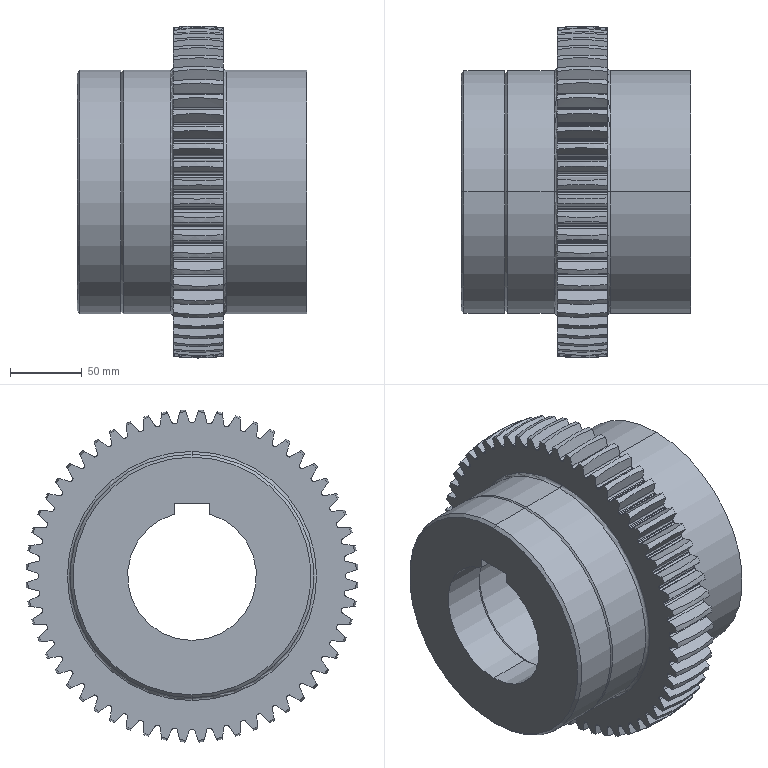Part | STEP file | External ring gear m=4  Z=56 | 1 solid | 391 faces | box 160.5 x 231.789 x 231.789 mm | volume 3084589 mm3 | cylinder 202 | spline 112 | sphere 56 | plane 10 | cone 7 | torus 4 | commonest cylinder face diameters 3.04 x136 214 x57 170 x6 90 x2 95 x1